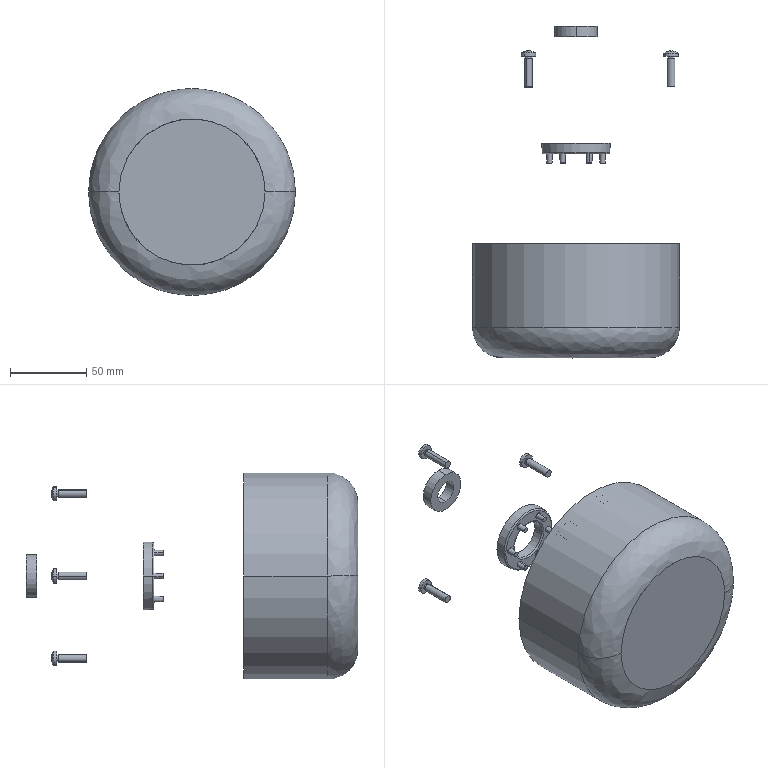Part | SolidWorks | 7 solids | 410 faces | box 136 x 218 x 136 mm | volume 125195 mm3 | plane 224 | cylinder 117 | spline 37 | cone 32 | commonest cylinder face diameters 2 x30 104 x11 64 x9 134 x9 116 x8 4.25 x6